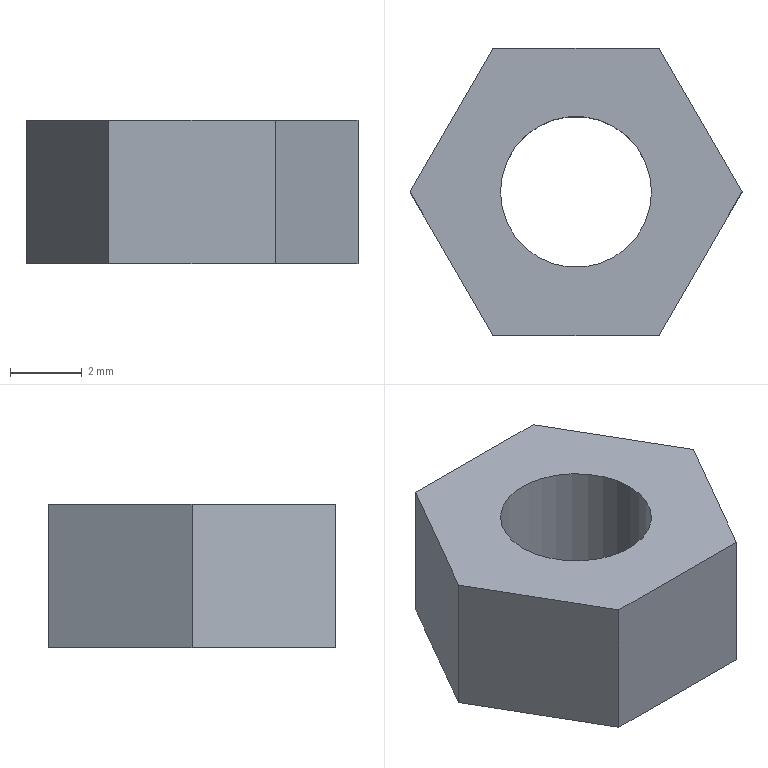Part | NX | 1 solid | 10 faces | box 9.238 x 8 x 4 mm | volume 166.285 mm3 | plane 8 | cylinder 2 | commonest cylinder face diameters 4.2 x2
STEP:
#1=CARTESIAN_POINT('',(2.309,4.,0.));
#2=VERTEX_POINT('',#1);
#3=CARTESIAN_POINT('',(4.619,0.,0.));
#4=VERTEX_POINT('',#3);
#5=CARTESIAN_POINT('',(2.309,4.,0.));
#6=DIRECTION('',(0.5,-0.866,0.));
#7=VECTOR('',#6,1000.);
#8=LINE('',#5,#7);
#9=EDGE_CURVE('',#2,#4,#8,.T.);
#10=ORIENTED_EDGE('',*,*,#9,.F.);
#11=CARTESIAN_POINT('',(-2.309,4.,0.));
#12=VERTEX_POINT('',#11);
#13=CARTESIAN_POINT('',(2.309,4.,0.));
#14=DIRECTION('',(-1.,0.,0.));
#15=VECTOR('',#14,1000.);
#16=LINE('',#13,#15);
#17=EDGE_CURVE('',#2,#12,#16,.T.);
#18=ORIENTED_EDGE('',*,*,#17,.T.);
#19=CARTESIAN_POINT('',(-4.619,0.,0.));
#20=VERTEX_POINT('',#19);
#21=CARTESIAN_POINT('',(-4.619,0.,0.));
#22=DIRECTION('',(0.5,0.866,0.));
#23=VECTOR('',#22,1000.);
#24=LINE('',#21,#23);
#25=EDGE_CURVE('',#20,#12,#24,.T.);
#26=ORIENTED_EDGE('',*,*,#25,.F.);
#27=CARTESIAN_POINT('',(-2.309,-4.,0.));
#28=VERTEX_POINT('',#27);
#29=CARTESIAN_POINT('',(-2.309,-4.,0.));
#30=DIRECTION('',(-0.5,0.866,0.));
#31=VECTOR('',#30,1000.);
#32=LINE('',#29,#31);
#33=EDGE_CURVE('',#28,#20,#32,.T.);
#34=ORIENTED_EDGE('',*,*,#33,.F.);
#35=CARTESIAN_POINT('',(2.309,-4.,0.));
#36=VERTEX_POINT('',#35);
#37=CARTESIAN_POINT('',(-2.309,-4.,0.));
#38=DIRECTION('',(1.,0.,0.));
#39=VECTOR('',#38,1000.);
#40=LINE('',#37,#39);
#41=EDGE_CURVE('',#28,#36,#40,.T.);
#42=ORIENTED_EDGE('',*,*,#41,.T.);
#43=CARTESIAN_POINT('',(4.619,0.,0.));
#44=DIRECTION('',(-0.5,-0.866,0.));
#45=VECTOR('',#44,1000.);
#46=LINE('',#43,#45);
#47=EDGE_CURVE('',#4,#36,#46,.T.);
#48=ORIENTED_EDGE('',*,*,#47,.F.);
#49=EDGE_LOOP('',(#10,#18,#26,#34,#42,#48));
#50=FACE_BOUND('',#49,.T.);
#51=CARTESIAN_POINT('',(-2.1,0.,0.));
#52=VERTEX_POINT('',#51);
#53=CARTESIAN_POINT('',(2.1,0.,0.));
#54=VERTEX_POINT('',#53);
#55=CARTESIAN_POINT('',(0.,0.,0.));
#56=DIRECTION('',(0.,0.,1.));
#57=DIRECTION('',(-1.,0.,0.));
#58=AXIS2_PLACEMENT_3D('',#55,#56,#57);
#59=CIRCLE('',#58,2.1);
#60=EDGE_CURVE('',#52,#54,#59,.T.);
#61=ORIENTED_EDGE('',*,*,#60,.F.);
#62=CARTESIAN_POINT('',(0.,0.,0.));
#63=DIRECTION('',(0.,0.,1.));
#64=DIRECTION('',(-1.,0.,0.));
#65=AXIS2_PLACEMENT_3D('',#62,#63,#64);
#66=CIRCLE('',#65,2.1);
#67=EDGE_CURVE('',#54,#52,#66,.T.);
#68=ORIENTED_EDGE('',*,*,#67,.F.);
#69=EDGE_LOOP('',(#61,#68));
#70=FACE_BOUND('',#69,.T.);
#71=CARTESIAN_POINT('',(0.,0.,0.));
#72=DIRECTION('',(0.,0.,-1.));
#73=DIRECTION('',(0.,-1.,0.));
#74=AXIS2_PLACEMENT_3D('',#71,#72,#73);
#75=PLANE('',#74);
#76=ADVANCED_FACE('',(#50,#70),#75,.F.);
#77=ORIENTED_EDGE('',*,*,#9,.T.);
#78=CARTESIAN_POINT('',(4.619,0.,-4.));
#79=VERTEX_POINT('',#78);
#80=CARTESIAN_POINT('',(4.619,0.,-4.));
#81=DIRECTION('',(0.,0.,1.));
#82=VECTOR('',#81,1000.);
#83=LINE('',#80,#82);
#84=EDGE_CURVE('',#79,#4,#83,.T.);
#85=ORIENTED_EDGE('',*,*,#84,.F.);
#86=CARTESIAN_POINT('',(2.309,4.,-4.));
#87=VERTEX_POINT('',#86);
#88=CARTESIAN_POINT('',(4.619,0.,-4.));
#89=DIRECTION('',(-0.5,0.866,0.));
#90=VECTOR('',#89,1000.);
#91=LINE('',#88,#90);
#92=EDGE_CURVE('',#79,#87,#91,.T.);
#93=ORIENTED_EDGE('',*,*,#92,.T.);
#94=CARTESIAN_POINT('',(2.309,4.,-4.));
#95=DIRECTION('',(0.,0.,1.));
#96=VECTOR('',#95,1000.);
#97=LINE('',#94,#96);
#98=EDGE_CURVE('',#87,#2,#97,.T.);
#99=ORIENTED_EDGE('',*,*,#98,.T.);
#100=EDGE_LOOP('',(#77,#85,#93,#99));
#101=FACE_BOUND('',#100,.T.);
#102=CARTESIAN_POINT('',(2.309,4.,0.));
#103=DIRECTION('',(0.866,0.5,0.));
#104=DIRECTION('',(0.,0.,-1.));
#105=AXIS2_PLACEMENT_3D('',#102,#103,#104);
#106=PLANE('',#105);
#107=ADVANCED_FACE('',(#101),#106,.T.);
#108=ORIENTED_EDGE('',*,*,#17,.F.);
#109=ORIENTED_EDGE('',*,*,#98,.F.);
#110=CARTESIAN_POINT('',(-2.309,4.,-4.));
#111=VERTEX_POINT('',#110);
#112=CARTESIAN_POINT('',(2.309,4.,-4.));
#113=DIRECTION('',(-1.,0.,0.));
#114=VECTOR('',#113,1000.);
#115=LINE('',#112,#114);
#116=EDGE_CURVE('',#87,#111,#115,.T.);
#117=ORIENTED_EDGE('',*,*,#116,.T.);
#118=CARTESIAN_POINT('',(-2.309,4.,-4.));
#119=DIRECTION('',(0.,0.,1.));
#120=VECTOR('',#119,1000.);
#121=LINE('',#118,#120);
#122=EDGE_CURVE('',#111,#12,#121,.T.);
#123=ORIENTED_EDGE('',*,*,#122,.T.);
#124=EDGE_LOOP('',(#108,#109,#117,#123));
#125=FACE_BOUND('',#124,.T.);
#126=CARTESIAN_POINT('',(-2.309,4.,0.));
#127=DIRECTION('',(0.,1.,0.));
#128=DIRECTION('',(1.,0.,0.));
#129=AXIS2_PLACEMENT_3D('',#126,#127,#128);
#130=PLANE('',#129);
#131=ADVANCED_FACE('',(#125),#130,.T.);
#132=ORIENTED_EDGE('',*,*,#25,.T.);
#133=ORIENTED_EDGE('',*,*,#122,.F.);
#134=CARTESIAN_POINT('',(-4.619,0.,-4.));
#135=VERTEX_POINT('',#134);
#136=CARTESIAN_POINT('',(-2.309,4.,-4.));
#137=DIRECTION('',(-0.5,-0.866,0.));
#138=VECTOR('',#137,1000.);
#139=LINE('',#136,#138);
#140=EDGE_CURVE('',#111,#135,#139,.T.);
#141=ORIENTED_EDGE('',*,*,#140,.T.);
#142=CARTESIAN_POINT('',(-4.619,0.,-4.));
#143=DIRECTION('',(0.,0.,1.));
#144=VECTOR('',#143,1000.);
#145=LINE('',#142,#144);
#146=EDGE_CURVE('',#135,#20,#145,.T.);
#147=ORIENTED_EDGE('',*,*,#146,.T.);
#148=EDGE_LOOP('',(#132,#133,#141,#147));
#149=FACE_BOUND('',#148,.T.);
#150=CARTESIAN_POINT('',(-4.619,0.,0.));
#151=DIRECTION('',(-0.866,0.5,0.));
#152=DIRECTION('',(0.,0.,1.));
#153=AXIS2_PLACEMENT_3D('',#150,#151,#152);
#154=PLANE('',#153);
#155=ADVANCED_FACE('',(#149),#154,.T.);
#156=ORIENTED_EDGE('',*,*,#33,.T.);
#157=ORIENTED_EDGE('',*,*,#146,.F.);
#158=CARTESIAN_POINT('',(-2.309,-4.,-4.));
#159=VERTEX_POINT('',#158);
#160=CARTESIAN_POINT('',(-4.619,0.,-4.));
#161=DIRECTION('',(0.5,-0.866,0.));
#162=VECTOR('',#161,1000.);
#163=LINE('',#160,#162);
#164=EDGE_CURVE('',#135,#159,#163,.T.);
#165=ORIENTED_EDGE('',*,*,#164,.T.);
#166=CARTESIAN_POINT('',(-2.309,-4.,-4.));
#167=DIRECTION('',(0.,0.,1.));
#168=VECTOR('',#167,1000.);
#169=LINE('',#166,#168);
#170=EDGE_CURVE('',#159,#28,#169,.T.);
#171=ORIENTED_EDGE('',*,*,#170,.T.);
#172=EDGE_LOOP('',(#156,#157,#165,#171));
#173=FACE_BOUND('',#172,.T.);
#174=CARTESIAN_POINT('',(-2.309,-4.,0.));
#175=DIRECTION('',(-0.866,-0.5,0.));
#176=DIRECTION('',(-0.5,0.866,0.));
#177=AXIS2_PLACEMENT_3D('',#174,#175,#176);
#178=PLANE('',#177);
#179=ADVANCED_FACE('',(#173),#178,.T.);
#180=ORIENTED_EDGE('',*,*,#41,.F.);
#181=ORIENTED_EDGE('',*,*,#170,.F.);
#182=CARTESIAN_POINT('',(2.309,-4.,-4.));
#183=VERTEX_POINT('',#182);
#184=CARTESIAN_POINT('',(-2.309,-4.,-4.));
#185=DIRECTION('',(1.,0.,0.));
#186=VECTOR('',#185,1000.);
#187=LINE('',#184,#186);
#188=EDGE_CURVE('',#159,#183,#187,.T.);
#189=ORIENTED_EDGE('',*,*,#188,.T.);
#190=CARTESIAN_POINT('',(2.309,-4.,-4.));
#191=DIRECTION('',(0.,0.,1.));
#192=VECTOR('',#191,1000.);
#193=LINE('',#190,#192);
#194=EDGE_CURVE('',#183,#36,#193,.T.);
#195=ORIENTED_EDGE('',*,*,#194,.T.);
#196=EDGE_LOOP('',(#180,#181,#189,#195));
#197=FACE_BOUND('',#196,.T.);
#198=CARTESIAN_POINT('',(2.309,-4.,0.));
#199=DIRECTION('',(0.,-1.,0.));
#200=DIRECTION('',(0.,0.,-1.));
#201=AXIS2_PLACEMENT_3D('',#198,#199,#200);
#202=PLANE('',#201);
#203=ADVANCED_FACE('',(#197),#202,.T.);
#204=ORIENTED_EDGE('',*,*,#47,.T.);
#205=ORIENTED_EDGE('',*,*,#194,.F.);
#206=CARTESIAN_POINT('',(2.309,-4.,-4.));
#207=DIRECTION('',(0.5,0.866,0.));
#208=VECTOR('',#207,1000.);
#209=LINE('',#206,#208);
#210=EDGE_CURVE('',#183,#79,#209,.T.);
#211=ORIENTED_EDGE('',*,*,#210,.T.);
#212=ORIENTED_EDGE('',*,*,#84,.T.);
#213=EDGE_LOOP('',(#204,#205,#211,#212));
#214=FACE_BOUND('',#213,.T.);
#215=CARTESIAN_POINT('',(4.619,0.,0.));
#216=DIRECTION('',(0.866,-0.5,0.));
#217=DIRECTION('',(0.,0.,-1.));
#218=AXIS2_PLACEMENT_3D('',#215,#216,#217);
#219=PLANE('',#218);
#220=ADVANCED_FACE('',(#214),#219,.T.);
#221=ORIENTED_EDGE('',*,*,#92,.F.);
#222=ORIENTED_EDGE('',*,*,#210,.F.);
#223=ORIENTED_EDGE('',*,*,#188,.F.);
#224=ORIENTED_EDGE('',*,*,#164,.F.);
#225=ORIENTED_EDGE('',*,*,#140,.F.);
#226=ORIENTED_EDGE('',*,*,#116,.F.);
#227=EDGE_LOOP('',(#221,#222,#223,#224,#225,#226));
#228=FACE_BOUND('',#227,.T.);
#229=CARTESIAN_POINT('',(-2.1,0.,-4.));
#230=VERTEX_POINT('',#229);
#231=CARTESIAN_POINT('',(2.1,0.,-4.));
#232=VERTEX_POINT('',#231);
#233=CARTESIAN_POINT('',(0.,0.,-4.));
#234=DIRECTION('',(0.,0.,-1.));
#235=DIRECTION('',(1.,0.,0.));
#236=AXIS2_PLACEMENT_3D('',#233,#234,#235);
#237=CIRCLE('',#236,2.1);
#238=EDGE_CURVE('',#230,#232,#237,.T.);
#239=ORIENTED_EDGE('',*,*,#238,.F.);
#240=CARTESIAN_POINT('',(0.,0.,-4.));
#241=DIRECTION('',(0.,0.,-1.));
#242=DIRECTION('',(1.,0.,0.));
#243=AXIS2_PLACEMENT_3D('',#240,#241,#242);
#244=CIRCLE('',#243,2.1);
#245=EDGE_CURVE('',#232,#230,#244,.T.);
#246=ORIENTED_EDGE('',*,*,#245,.F.);
#247=EDGE_LOOP('',(#239,#246));
#248=FACE_BOUND('',#247,.T.);
#249=CARTESIAN_POINT('',(0.,0.,-4.));
#250=DIRECTION('',(0.,0.,-1.));
#251=DIRECTION('',(0.,-1.,0.));
#252=AXIS2_PLACEMENT_3D('',#249,#250,#251);
#253=PLANE('',#252);
#254=ADVANCED_FACE('',(#228,#248),#253,.T.);
#255=ORIENTED_EDGE('',*,*,#60,.T.);
#256=CARTESIAN_POINT('',(2.1,0.,-4.));
#257=DIRECTION('',(0.,0.,1.));
#258=VECTOR('',#257,1000.);
#259=LINE('',#256,#258);
#260=EDGE_CURVE('',#232,#54,#259,.T.);
#261=ORIENTED_EDGE('',*,*,#260,.F.);
#262=ORIENTED_EDGE('',*,*,#245,.T.);
#263=CARTESIAN_POINT('',(-2.1,0.,-4.));
#264=DIRECTION('',(0.,0.,1.));
#265=VECTOR('',#264,1000.);
#266=LINE('',#263,#265);
#267=EDGE_CURVE('',#230,#52,#266,.T.);
#268=ORIENTED_EDGE('',*,*,#267,.T.);
#269=EDGE_LOOP('',(#255,#261,#262,#268));
#270=FACE_BOUND('',#269,.T.);
#271=CARTESIAN_POINT('',(0.,0.,-4.));
#272=DIRECTION('',(0.,0.,1.));
#273=DIRECTION('',(1.,0.,0.));
#274=AXIS2_PLACEMENT_3D('',#271,#272,#273);
#275=CYLINDRICAL_SURFACE('',#274,2.1);
#276=ADVANCED_FACE('',(#270),#275,.F.);
#277=ORIENTED_EDGE('',*,*,#238,.T.);
#278=ORIENTED_EDGE('',*,*,#260,.T.);
#279=ORIENTED_EDGE('',*,*,#67,.T.);
#280=ORIENTED_EDGE('',*,*,#267,.F.);
#281=EDGE_LOOP('',(#277,#278,#279,#280));
#282=FACE_BOUND('',#281,.T.);
#283=CARTESIAN_POINT('',(0.,0.,-4.));
#284=DIRECTION('',(0.,0.,1.));
#285=DIRECTION('',(1.,0.,0.));
#286=AXIS2_PLACEMENT_3D('',#283,#284,#285);
#287=CYLINDRICAL_SURFACE('',#286,2.1);
#288=ADVANCED_FACE('',(#282),#287,.F.);
#289=CLOSED_SHELL('',(#76,#107,#131,#155,#179,#203,#220,#254,#276,#288));
#290=MANIFOLD_SOLID_BREP('',#289);
#291=(LENGTH_UNIT()NAMED_UNIT(*)SI_UNIT(.MILLI.,.METRE.));
#292=UNCERTAINTY_MEASURE_WITH_UNIT(LENGTH_MEASURE(0.00001),#291,'','');
#293=(NAMED_UNIT(*)PLANE_ANGLE_UNIT()SI_UNIT($,.RADIAN.));
#294=(NAMED_UNIT(*)SI_UNIT($,.STERADIAN.)SOLID_ANGLE_UNIT());
#295=(GEOMETRIC_REPRESENTATION_CONTEXT(3)GLOBAL_UNCERTAINTY_ASSIGNED_CONTEXT((#292))GLOBAL_UNIT_ASSIGNED_CONTEXT((#291,#293,#294))REPRESENTATION_CONTEXT('',''));
#296=ADVANCED_BREP_SHAPE_REPRESENTATION('',(#290),#295);